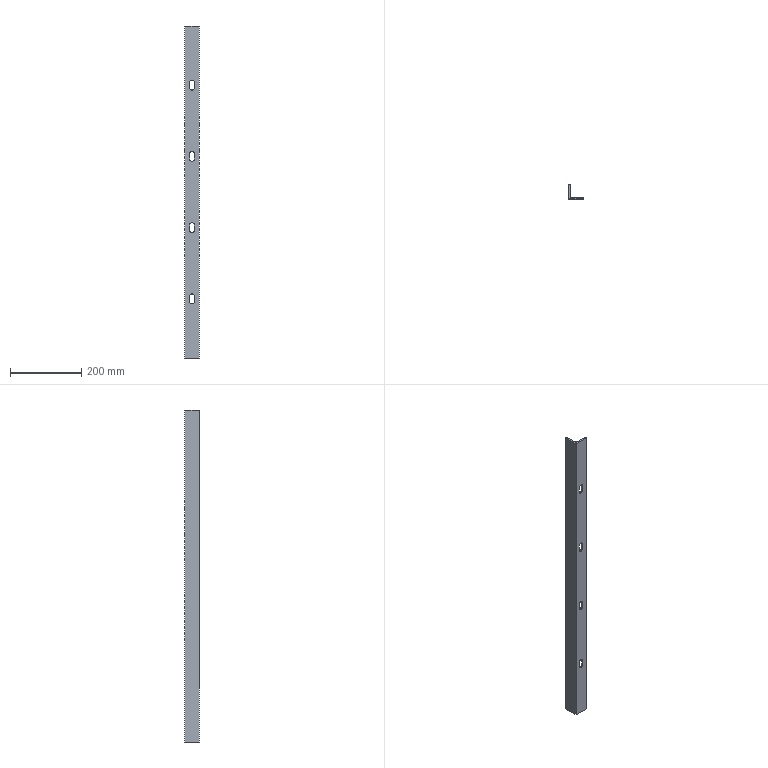Part | SolidWorks | features BaseBody 1 | 1 solid | 27 faces | box 40 x 40 x 932 mm | volume 282373 mm3 | plane 16 | cylinder 11 | commonest cylinder face diameters 13 x8 2.667 x2 10 x1
STEP:
#1=CARTESIAN_POINT('',(-11.3,51.3,0.));
#2=VERTEX_POINT('',#1);
#3=CARTESIAN_POINT('',(-11.3,11.3,0.));
#4=VERTEX_POINT('',#3);
#5=CARTESIAN_POINT('',(-11.3,11.3,0.));
#6=DIRECTION('',(0.,-1.,0.));
#7=VECTOR('',#6,1000.);
#8=LINE('',#5,#7);
#9=EDGE_CURVE('',#2,#4,#8,.T.);
#10=ORIENTED_EDGE('',*,*,#9,.T.);
#11=CARTESIAN_POINT('',(-11.3,11.3,932.));
#12=VERTEX_POINT('',#11);
#13=CARTESIAN_POINT('',(-11.3,11.3,0.));
#14=DIRECTION('',(0.,0.,1.));
#15=VECTOR('',#14,1000.);
#16=LINE('',#13,#15);
#17=EDGE_CURVE('',#4,#12,#16,.T.);
#18=ORIENTED_EDGE('',*,*,#17,.T.);
#19=CARTESIAN_POINT('',(-11.3,51.3,932.));
#20=VERTEX_POINT('',#19);
#21=CARTESIAN_POINT('',(-11.3,11.3,932.));
#22=DIRECTION('',(0.,1.,0.));
#23=VECTOR('',#22,1000.);
#24=LINE('',#21,#23);
#25=EDGE_CURVE('',#12,#20,#24,.T.);
#26=ORIENTED_EDGE('',*,*,#25,.T.);
#27=CARTESIAN_POINT('',(-11.3,51.3,0.));
#28=DIRECTION('',(0.,0.,-1.));
#29=VECTOR('',#28,1000.);
#30=LINE('',#27,#29);
#31=EDGE_CURVE('',#20,#2,#30,.T.);
#32=ORIENTED_EDGE('',*,*,#31,.T.);
#33=EDGE_LOOP('',(#10,#18,#26,#32));
#34=FACE_OUTER_BOUND('',#33,.T.);
#35=CARTESIAN_POINT('',(-11.3,11.3,0.));
#36=DIRECTION('',(-1.,0.,0.));
#37=DIRECTION('',(0.,-1.,0.));
#38=AXIS2_PLACEMENT_3D('',#35,#36,#37);
#39=PLANE('',#38);
#40=ADVANCED_FACE('',(#34),#39,.T.);
#41=CARTESIAN_POINT('',(2.2,11.3,773.5));
#42=VERTEX_POINT('',#41);
#43=CARTESIAN_POINT('',(15.2,11.3,773.5));
#44=VERTEX_POINT('',#43);
#45=CARTESIAN_POINT('',(8.7,11.3,773.5));
#46=DIRECTION('',(0.,1.,0.));
#47=DIRECTION('',(-1.,0.,0.));
#48=AXIS2_PLACEMENT_3D('',#45,#46,#47);
#49=CIRCLE('',#48,6.5);
#50=EDGE_CURVE('',#42,#44,#49,.T.);
#51=ORIENTED_EDGE('',*,*,#50,.T.);
#52=CARTESIAN_POINT('',(15.2,11.3,758.5));
#53=VERTEX_POINT('',#52);
#54=CARTESIAN_POINT('',(15.2,11.3,0.));
#55=DIRECTION('',(0.,0.,-1.));
#56=VECTOR('',#55,1000.);
#57=LINE('',#54,#56);
#58=EDGE_CURVE('',#44,#53,#57,.T.);
#59=ORIENTED_EDGE('',*,*,#58,.T.);
#60=CARTESIAN_POINT('',(2.2,11.3,758.5));
#61=VERTEX_POINT('',#60);
#62=CARTESIAN_POINT('',(8.7,11.3,758.5));
#63=DIRECTION('',(0.,1.,0.));
#64=DIRECTION('',(-1.,0.,0.));
#65=AXIS2_PLACEMENT_3D('',#62,#63,#64);
#66=CIRCLE('',#65,6.5);
#67=EDGE_CURVE('',#53,#61,#66,.T.);
#68=ORIENTED_EDGE('',*,*,#67,.T.);
#69=CARTESIAN_POINT('',(2.2,11.3,0.));
#70=DIRECTION('',(0.,0.,1.));
#71=VECTOR('',#70,1000.);
#72=LINE('',#69,#71);
#73=EDGE_CURVE('',#61,#42,#72,.T.);
#74=ORIENTED_EDGE('',*,*,#73,.T.);
#75=EDGE_LOOP('',(#51,#59,#68,#74));
#76=FACE_BOUND('',#75,.T.);
#77=CARTESIAN_POINT('',(2.2,11.3,573.5));
#78=VERTEX_POINT('',#77);
#79=CARTESIAN_POINT('',(15.2,11.3,573.5));
#80=VERTEX_POINT('',#79);
#81=CARTESIAN_POINT('',(8.7,11.3,573.5));
#82=DIRECTION('',(0.,1.,0.));
#83=DIRECTION('',(-1.,0.,0.));
#84=AXIS2_PLACEMENT_3D('',#81,#82,#83);
#85=CIRCLE('',#84,6.5);
#86=EDGE_CURVE('',#78,#80,#85,.T.);
#87=ORIENTED_EDGE('',*,*,#86,.T.);
#88=CARTESIAN_POINT('',(15.2,11.3,558.5));
#89=VERTEX_POINT('',#88);
#90=CARTESIAN_POINT('',(15.2,11.3,0.));
#91=DIRECTION('',(0.,0.,-1.));
#92=VECTOR('',#91,1000.);
#93=LINE('',#90,#92);
#94=EDGE_CURVE('',#80,#89,#93,.T.);
#95=ORIENTED_EDGE('',*,*,#94,.T.);
#96=CARTESIAN_POINT('',(2.2,11.3,558.5));
#97=VERTEX_POINT('',#96);
#98=CARTESIAN_POINT('',(8.7,11.3,558.5));
#99=DIRECTION('',(0.,1.,0.));
#100=DIRECTION('',(-1.,0.,0.));
#101=AXIS2_PLACEMENT_3D('',#98,#99,#100);
#102=CIRCLE('',#101,6.5);
#103=EDGE_CURVE('',#89,#97,#102,.T.);
#104=ORIENTED_EDGE('',*,*,#103,.T.);
#105=CARTESIAN_POINT('',(2.2,11.3,0.));
#106=DIRECTION('',(0.,0.,1.));
#107=VECTOR('',#106,1000.);
#108=LINE('',#105,#107);
#109=EDGE_CURVE('',#97,#78,#108,.T.);
#110=ORIENTED_EDGE('',*,*,#109,.T.);
#111=EDGE_LOOP('',(#87,#95,#104,#110));
#112=FACE_BOUND('',#111,.T.);
#113=CARTESIAN_POINT('',(2.2,11.3,373.5));
#114=VERTEX_POINT('',#113);
#115=CARTESIAN_POINT('',(15.2,11.3,373.5));
#116=VERTEX_POINT('',#115);
#117=CARTESIAN_POINT('',(8.7,11.3,373.5));
#118=DIRECTION('',(0.,1.,0.));
#119=DIRECTION('',(-1.,0.,0.));
#120=AXIS2_PLACEMENT_3D('',#117,#118,#119);
#121=CIRCLE('',#120,6.5);
#122=EDGE_CURVE('',#114,#116,#121,.T.);
#123=ORIENTED_EDGE('',*,*,#122,.T.);
#124=CARTESIAN_POINT('',(15.2,11.3,358.5));
#125=VERTEX_POINT('',#124);
#126=CARTESIAN_POINT('',(15.2,11.3,0.));
#127=DIRECTION('',(0.,0.,-1.));
#128=VECTOR('',#127,1000.);
#129=LINE('',#126,#128);
#130=EDGE_CURVE('',#116,#125,#129,.T.);
#131=ORIENTED_EDGE('',*,*,#130,.T.);
#132=CARTESIAN_POINT('',(2.2,11.3,358.5));
#133=VERTEX_POINT('',#132);
#134=CARTESIAN_POINT('',(8.7,11.3,358.5));
#135=DIRECTION('',(0.,1.,0.));
#136=DIRECTION('',(-1.,0.,0.));
#137=AXIS2_PLACEMENT_3D('',#134,#135,#136);
#138=CIRCLE('',#137,6.5);
#139=EDGE_CURVE('',#125,#133,#138,.T.);
#140=ORIENTED_EDGE('',*,*,#139,.T.);
#141=CARTESIAN_POINT('',(2.2,11.3,0.));
#142=DIRECTION('',(0.,0.,1.));
#143=VECTOR('',#142,1000.);
#144=LINE('',#141,#143);
#145=EDGE_CURVE('',#133,#114,#144,.T.);
#146=ORIENTED_EDGE('',*,*,#145,.T.);
#147=EDGE_LOOP('',(#123,#131,#140,#146));
#148=FACE_BOUND('',#147,.T.);
#149=CARTESIAN_POINT('',(2.2,11.3,173.5));
#150=VERTEX_POINT('',#149);
#151=CARTESIAN_POINT('',(15.2,11.3,173.5));
#152=VERTEX_POINT('',#151);
#153=CARTESIAN_POINT('',(8.7,11.3,173.5));
#154=DIRECTION('',(0.,1.,0.));
#155=DIRECTION('',(-1.,0.,0.));
#156=AXIS2_PLACEMENT_3D('',#153,#154,#155);
#157=CIRCLE('',#156,6.5);
#158=EDGE_CURVE('',#150,#152,#157,.T.);
#159=ORIENTED_EDGE('',*,*,#158,.T.);
#160=CARTESIAN_POINT('',(15.2,11.3,158.5));
#161=VERTEX_POINT('',#160);
#162=CARTESIAN_POINT('',(15.2,11.3,0.));
#163=DIRECTION('',(0.,0.,-1.));
#164=VECTOR('',#163,1000.);
#165=LINE('',#162,#164);
#166=EDGE_CURVE('',#152,#161,#165,.T.);
#167=ORIENTED_EDGE('',*,*,#166,.T.);
#168=CARTESIAN_POINT('',(2.2,11.3,158.5));
#169=VERTEX_POINT('',#168);
#170=CARTESIAN_POINT('',(8.7,11.3,158.5));
#171=DIRECTION('',(0.,1.,0.));
#172=DIRECTION('',(-1.,0.,0.));
#173=AXIS2_PLACEMENT_3D('',#170,#171,#172);
#174=CIRCLE('',#173,6.5);
#175=EDGE_CURVE('',#161,#169,#174,.T.);
#176=ORIENTED_EDGE('',*,*,#175,.T.);
#177=CARTESIAN_POINT('',(2.2,11.3,0.));
#178=DIRECTION('',(0.,0.,1.));
#179=VECTOR('',#178,1000.);
#180=LINE('',#177,#179);
#181=EDGE_CURVE('',#169,#150,#180,.T.);
#182=ORIENTED_EDGE('',*,*,#181,.T.);
#183=EDGE_LOOP('',(#159,#167,#176,#182));
#184=FACE_BOUND('',#183,.T.);
#185=CARTESIAN_POINT('',(28.7,11.3,0.));
#186=VERTEX_POINT('',#185);
#187=CARTESIAN_POINT('',(28.7,11.3,0.));
#188=DIRECTION('',(1.,0.,0.));
#189=VECTOR('',#188,1000.);
#190=LINE('',#187,#189);
#191=EDGE_CURVE('',#4,#186,#190,.T.);
#192=ORIENTED_EDGE('',*,*,#191,.T.);
#193=CARTESIAN_POINT('',(28.7,11.3,932.));
#194=VERTEX_POINT('',#193);
#195=CARTESIAN_POINT('',(28.7,11.3,0.));
#196=DIRECTION('',(0.,0.,1.));
#197=VECTOR('',#196,1000.);
#198=LINE('',#195,#197);
#199=EDGE_CURVE('',#186,#194,#198,.T.);
#200=ORIENTED_EDGE('',*,*,#199,.T.);
#201=CARTESIAN_POINT('',(28.7,11.3,932.));
#202=DIRECTION('',(-1.,0.,0.));
#203=VECTOR('',#202,1000.);
#204=LINE('',#201,#203);
#205=EDGE_CURVE('',#194,#12,#204,.T.);
#206=ORIENTED_EDGE('',*,*,#205,.T.);
#207=ORIENTED_EDGE('',*,*,#17,.F.);
#208=EDGE_LOOP('',(#192,#200,#206,#207));
#209=FACE_OUTER_BOUND('',#208,.T.);
#210=CARTESIAN_POINT('',(28.7,11.3,0.));
#211=DIRECTION('',(0.,-1.,0.));
#212=DIRECTION('',(1.,0.,0.));
#213=AXIS2_PLACEMENT_3D('',#210,#211,#212);
#214=PLANE('',#213);
#215=ADVANCED_FACE('',(#76,#112,#148,#184,#209),#214,.T.);
#216=CARTESIAN_POINT('',(-8.633,51.3,0.));
#217=VERTEX_POINT('',#216);
#218=CARTESIAN_POINT('',(8.7,51.3,0.));
#219=DIRECTION('',(-1.,0.,0.));
#220=VECTOR('',#219,1000.);
#221=LINE('',#218,#220);
#222=EDGE_CURVE('',#217,#2,#221,.T.);
#223=ORIENTED_EDGE('',*,*,#222,.F.);
#224=CARTESIAN_POINT('',(-7.3,49.967,0.));
#225=VERTEX_POINT('',#224);
#226=CARTESIAN_POINT('',(-8.633,49.967,0.));
#227=DIRECTION('',(0.,0.,1.));
#228=DIRECTION('',(1.,0.,0.));
#229=AXIS2_PLACEMENT_3D('',#226,#227,#228);
#230=CIRCLE('',#229,1.333);
#231=EDGE_CURVE('',#225,#217,#230,.T.);
#232=ORIENTED_EDGE('',*,*,#231,.F.);
#233=CARTESIAN_POINT('',(-7.3,20.3,0.));
#234=VERTEX_POINT('',#233);
#235=CARTESIAN_POINT('',(-7.3,31.3,0.));
#236=DIRECTION('',(0.,1.,0.));
#237=VECTOR('',#236,1000.);
#238=LINE('',#235,#237);
#239=EDGE_CURVE('',#234,#225,#238,.T.);
#240=ORIENTED_EDGE('',*,*,#239,.F.);
#241=CARTESIAN_POINT('',(-2.3,15.3,0.));
#242=VERTEX_POINT('',#241);
#243=CARTESIAN_POINT('',(-2.3,20.3,0.));
#244=DIRECTION('',(0.,0.,-1.));
#245=DIRECTION('',(1.,0.,0.));
#246=AXIS2_PLACEMENT_3D('',#243,#244,#245);
#247=CIRCLE('',#246,5.);
#248=EDGE_CURVE('',#242,#234,#247,.T.);
#249=ORIENTED_EDGE('',*,*,#248,.F.);
#250=CARTESIAN_POINT('',(27.367,15.3,0.));
#251=VERTEX_POINT('',#250);
#252=CARTESIAN_POINT('',(8.7,15.3,0.));
#253=DIRECTION('',(-1.,0.,0.));
#254=VECTOR('',#253,1000.);
#255=LINE('',#252,#254);
#256=EDGE_CURVE('',#251,#242,#255,.T.);
#257=ORIENTED_EDGE('',*,*,#256,.F.);
#258=CARTESIAN_POINT('',(28.7,13.967,0.));
#259=VERTEX_POINT('',#258);
#260=CARTESIAN_POINT('',(27.367,13.967,0.));
#261=DIRECTION('',(0.,0.,1.));
#262=DIRECTION('',(1.,0.,0.));
#263=AXIS2_PLACEMENT_3D('',#260,#261,#262);
#264=CIRCLE('',#263,1.333);
#265=EDGE_CURVE('',#259,#251,#264,.T.);
#266=ORIENTED_EDGE('',*,*,#265,.F.);
#267=CARTESIAN_POINT('',(28.7,31.3,0.));
#268=DIRECTION('',(0.,1.,0.));
#269=VECTOR('',#268,1000.);
#270=LINE('',#267,#269);
#271=EDGE_CURVE('',#186,#259,#270,.T.);
#272=ORIENTED_EDGE('',*,*,#271,.F.);
#273=ORIENTED_EDGE('',*,*,#191,.F.);
#274=ORIENTED_EDGE('',*,*,#9,.F.);
#275=EDGE_LOOP('',(#223,#232,#240,#249,#257,#266,#272,#273,#274));
#276=FACE_OUTER_BOUND('',#275,.T.);
#277=CARTESIAN_POINT('',(8.7,31.3,0.));
#278=DIRECTION('',(0.,0.,1.));
#279=DIRECTION('',(1.,0.,0.));
#280=AXIS2_PLACEMENT_3D('',#277,#278,#279);
#281=PLANE('',#280);
#282=ADVANCED_FACE('',(#276),#281,.F.);
#283=ORIENTED_EDGE('',*,*,#222,.T.);
#284=ORIENTED_EDGE('',*,*,#31,.F.);
#285=CARTESIAN_POINT('',(-8.633,51.3,932.));
#286=VERTEX_POINT('',#285);
#287=CARTESIAN_POINT('',(-11.3,51.3,932.));
#288=DIRECTION('',(1.,0.,0.));
#289=VECTOR('',#288,1000.);
#290=LINE('',#287,#289);
#291=EDGE_CURVE('',#20,#286,#290,.T.);
#292=ORIENTED_EDGE('',*,*,#291,.T.);
#293=CARTESIAN_POINT('',(-8.633,51.3,0.));
#294=DIRECTION('',(0.,0.,-1.));
#295=VECTOR('',#294,1000.);
#296=LINE('',#293,#295);
#297=EDGE_CURVE('',#286,#217,#296,.T.);
#298=ORIENTED_EDGE('',*,*,#297,.T.);
#299=EDGE_LOOP('',(#283,#284,#292,#298));
#300=FACE_OUTER_BOUND('',#299,.T.);
#301=CARTESIAN_POINT('',(-11.3,51.3,0.));
#302=DIRECTION('',(0.,1.,0.));
#303=DIRECTION('',(0.,0.,1.));
#304=AXIS2_PLACEMENT_3D('',#301,#302,#303);
#305=PLANE('',#304);
#306=ADVANCED_FACE('',(#300),#305,.T.);
#307=CARTESIAN_POINT('',(-7.3,49.967,932.));
#308=VERTEX_POINT('',#307);
#309=CARTESIAN_POINT('',(-8.633,49.967,932.));
#310=DIRECTION('',(0.,0.,1.));
#311=DIRECTION('',(1.,0.,0.));
#312=AXIS2_PLACEMENT_3D('',#309,#310,#311);
#313=CIRCLE('',#312,1.333);
#314=EDGE_CURVE('',#308,#286,#313,.T.);
#315=ORIENTED_EDGE('',*,*,#314,.T.);
#316=ORIENTED_EDGE('',*,*,#291,.F.);
#317=ORIENTED_EDGE('',*,*,#25,.F.);
#318=ORIENTED_EDGE('',*,*,#205,.F.);
#319=CARTESIAN_POINT('',(28.7,13.967,932.));
#320=VERTEX_POINT('',#319);
#321=CARTESIAN_POINT('',(28.7,31.3,932.));
#322=DIRECTION('',(0.,1.,0.));
#323=VECTOR('',#322,1000.);
#324=LINE('',#321,#323);
#325=EDGE_CURVE('',#194,#320,#324,.T.);
#326=ORIENTED_EDGE('',*,*,#325,.T.);
#327=CARTESIAN_POINT('',(27.367,15.3,932.));
#328=VERTEX_POINT('',#327);
#329=CARTESIAN_POINT('',(27.367,13.967,932.));
#330=DIRECTION('',(0.,0.,1.));
#331=DIRECTION('',(1.,0.,0.));
#332=AXIS2_PLACEMENT_3D('',#329,#330,#331);
#333=CIRCLE('',#332,1.333);
#334=EDGE_CURVE('',#320,#328,#333,.T.);
#335=ORIENTED_EDGE('',*,*,#334,.T.);
#336=CARTESIAN_POINT('',(-2.3,15.3,932.));
#337=VERTEX_POINT('',#336);
#338=CARTESIAN_POINT('',(8.7,15.3,932.));
#339=DIRECTION('',(-1.,0.,0.));
#340=VECTOR('',#339,1000.);
#341=LINE('',#338,#340);
#342=EDGE_CURVE('',#328,#337,#341,.T.);
#343=ORIENTED_EDGE('',*,*,#342,.T.);
#344=CARTESIAN_POINT('',(-7.3,20.3,932.));
#345=VERTEX_POINT('',#344);
#346=CARTESIAN_POINT('',(-2.3,20.3,932.));
#347=DIRECTION('',(0.,0.,-1.));
#348=DIRECTION('',(1.,0.,0.));
#349=AXIS2_PLACEMENT_3D('',#346,#347,#348);
#350=CIRCLE('',#349,5.);
#351=EDGE_CURVE('',#337,#345,#350,.T.);
#352=ORIENTED_EDGE('',*,*,#351,.T.);
#353=CARTESIAN_POINT('',(-7.3,31.3,932.));
#354=DIRECTION('',(0.,1.,0.));
#355=VECTOR('',#354,1000.);
#356=LINE('',#353,#355);
#357=EDGE_CURVE('',#345,#308,#356,.T.);
#358=ORIENTED_EDGE('',*,*,#357,.T.);
#359=EDGE_LOOP('',(#315,#316,#317,#318,#326,#335,#343,#352,#358));
#360=FACE_OUTER_BOUND('',#359,.T.);
#361=CARTESIAN_POINT('',(8.7,31.3,932.));
#362=DIRECTION('',(0.,0.,1.));
#363=DIRECTION('',(1.,0.,0.));
#364=AXIS2_PLACEMENT_3D('',#361,#362,#363);
#365=PLANE('',#364);
#366=ADVANCED_FACE('',(#360),#365,.T.);
#367=CARTESIAN_POINT('',(15.2,15.3,758.5));
#368=VERTEX_POINT('',#367);
#369=CARTESIAN_POINT('',(15.2,11.3,758.5));
#370=DIRECTION('',(0.,1.,0.));
#371=VECTOR('',#370,1000.);
#372=LINE('',#369,#371);
#373=EDGE_CURVE('',#53,#368,#372,.T.);
#374=ORIENTED_EDGE('',*,*,#373,.F.);
#375=ORIENTED_EDGE('',*,*,#58,.F.);
#376=CARTESIAN_POINT('',(15.2,15.3,773.5));
#377=VERTEX_POINT('',#376);
#378=CARTESIAN_POINT('',(15.2,11.3,773.5));
#379=DIRECTION('',(0.,-1.,0.));
#380=VECTOR('',#379,1000.);
#381=LINE('',#378,#380);
#382=EDGE_CURVE('',#377,#44,#381,.T.);
#383=ORIENTED_EDGE('',*,*,#382,.F.);
#384=CARTESIAN_POINT('',(15.2,15.3,773.5));
#385=DIRECTION('',(0.,0.,1.));
#386=VECTOR('',#385,1000.);
#387=LINE('',#384,#386);
#388=EDGE_CURVE('',#368,#377,#387,.T.);
#389=ORIENTED_EDGE('',*,*,#388,.F.);
#390=EDGE_LOOP('',(#374,#375,#383,#389));
#391=FACE_OUTER_BOUND('',#390,.T.);
#392=CARTESIAN_POINT('',(15.2,11.3,773.5));
#393=DIRECTION('',(1.,0.,0.));
#394=DIRECTION('',(0.,1.,0.));
#395=AXIS2_PLACEMENT_3D('',#392,#393,#394);
#396=PLANE('',#395);
#397=ADVANCED_FACE('',(#391),#396,.F.);
#398=ORIENTED_EDGE('',*,*,#382,.T.);
#399=ORIENTED_EDGE('',*,*,#50,.F.);
#400=CARTESIAN_POINT('',(2.2,15.3,773.5));
#401=VERTEX_POINT('',#400);
#402=CARTESIAN_POINT('',(2.2,11.3,773.5));
#403=DIRECTION('',(0.,-1.,0.));
#404=VECTOR('',#403,1000.);
#405=LINE('',#402,#404);
#406=EDGE_CURVE('',#401,#42,#405,.T.);
#407=ORIENTED_EDGE('',*,*,#406,.F.);
#408=CARTESIAN_POINT('',(8.7,15.3,773.5));
#409=DIRECTION('',(0.,-1.,0.));
#410=DIRECTION('',(-1.,0.,0.));
#411=AXIS2_PLACEMENT_3D('',#408,#409,#410);
#412=CIRCLE('',#411,6.5);
#413=EDGE_CURVE('',#377,#401,#412,.T.);
#414=ORIENTED_EDGE('',*,*,#413,.F.);
#415=EDGE_LOOP('',(#398,#399,#407,#414));
#416=FACE_OUTER_BOUND('',#415,.T.);
#417=CARTESIAN_POINT('',(8.7,11.3,773.5));
#418=DIRECTION('',(0.,1.,0.));
#419=DIRECTION('',(-1.,0.,0.));
#420=AXIS2_PLACEMENT_3D('',#417,#418,#419);
#421=CYLINDRICAL_SURFACE('',#420,6.5);
#422=ADVANCED_FACE('',(#416),#421,.F.);
#423=ORIENTED_EDGE('',*,*,#406,.T.);
#424=ORIENTED_EDGE('',*,*,#73,.F.);
#425=CARTESIAN_POINT('',(2.2,15.3,758.5));
#426=VERTEX_POINT('',#425);
#427=CARTESIAN_POINT('',(2.2,11.3,758.5));
#428=DIRECTION('',(0.,-1.,0.));
#429=VECTOR('',#428,1000.);
#430=LINE('',#427,#429);
#431=EDGE_CURVE('',#426,#61,#430,.T.);
#432=ORIENTED_EDGE('',*,*,#431,.F.);
#433=CARTESIAN_POINT('',(2.2,15.3,758.5));
#434=DIRECTION('',(0.,0.,-1.));
#435=VECTOR('',#434,1000.);
#436=LINE('',#433,#435);
#437=EDGE_CURVE('',#401,#426,#436,.T.);
#438=ORIENTED_EDGE('',*,*,#437,.F.);
#439=EDGE_LOOP('',(#423,#424,#432,#438));
#440=FACE_OUTER_BOUND('',#439,.T.);
#441=CARTESIAN_POINT('',(2.2,11.3,758.5));
#442=DIRECTION('',(-1.,0.,0.));
#443=DIRECTION('',(0.,0.,1.));
#444=AXIS2_PLACEMENT_3D('',#441,#442,#443);
#445=PLANE('',#444);
#446=ADVANCED_FACE('',(#440),#445,.F.);
#447=ORIENTED_EDGE('',*,*,#431,.T.);
#448=ORIENTED_EDGE('',*,*,#67,.F.);
#449=ORIENTED_EDGE('',*,*,#373,.T.);
#450=CARTESIAN_POINT('',(8.7,15.3,758.5));
#451=DIRECTION('',(0.,-1.,0.));
#452=DIRECTION('',(-1.,0.,0.));
#453=AXIS2_PLACEMENT_3D('',#450,#451,#452);
#454=CIRCLE('',#453,6.5);
#455=EDGE_CURVE('',#426,#368,#454,.T.);
#456=ORIENTED_EDGE('',*,*,#455,.F.);
#457=EDGE_LOOP('',(#447,#448,#449,#456));
#458=FACE_OUTER_BOUND('',#457,.T.);
#459=CARTESIAN_POINT('',(8.7,11.3,758.5));
#460=DIRECTION('',(0.,1.,0.));
#461=DIRECTION('',(-1.,0.,0.));
#462=AXIS2_PLACEMENT_3D('',#459,#460,#461);
#463=CYLINDRICAL_SURFACE('',#462,6.5);
#464=ADVANCED_FACE('',(#458),#463,.F.);
#465=CARTESIAN_POINT('',(15.2,15.3,558.5));
#466=VERTEX_POINT('',#465);
#467=CARTESIAN_POINT('',(15.2,11.3,558.5));
#468=DIRECTION('',(0.,1.,0.));
#469=VECTOR('',#468,1000.);
#470=LINE('',#467,#469);
#471=EDGE_CURVE('',#89,#466,#470,.T.);
#472=ORIENTED_EDGE('',*,*,#471,.F.);
#473=ORIENTED_EDGE('',*,*,#94,.F.);
#474=CARTESIAN_POINT('',(15.2,15.3,573.5));
#475=VERTEX_POINT('',#474);
#476=CARTESIAN_POINT('',(15.2,11.3,573.5));
#477=DIRECTION('',(0.,-1.,0.));
#478=VECTOR('',#477,1000.);
#479=LINE('',#476,#478);
#480=EDGE_CURVE('',#475,#80,#479,.T.);
#481=ORIENTED_EDGE('',*,*,#480,.F.);
#482=CARTESIAN_POINT('',(15.2,15.3,573.5));
#483=DIRECTION('',(0.,0.,1.));
#484=VECTOR('',#483,1000.);
#485=LINE('',#482,#484);
#486=EDGE_CURVE('',#466,#475,#485,.T.);
#487=ORIENTED_EDGE('',*,*,#486,.F.);
#488=EDGE_LOOP('',(#472,#473,#481,#487));
#489=FACE_OUTER_BOUND('',#488,.T.);
#490=CARTESIAN_POINT('',(15.2,11.3,573.5));
#491=DIRECTION('',(1.,0.,0.));
#492=DIRECTION('',(0.,1.,0.));
#493=AXIS2_PLACEMENT_3D('',#490,#491,#492);
#494=PLANE('',#493);
#495=ADVANCED_FACE('',(#489),#494,.F.);
#496=ORIENTED_EDGE('',*,*,#480,.T.);
#497=ORIENTED_EDGE('',*,*,#86,.F.);
#498=CARTESIAN_POINT('',(2.2,15.3,573.5));
#499=VERTEX_POINT('',#498);
#500=CARTESIAN_POINT('',(2.2,11.3,573.5));
#501=DIRECTION('',(0.,-1.,0.));
#502=VECTOR('',#501,1000.);
#503=LINE('',#500,#502);
#504=EDGE_CURVE('',#499,#78,#503,.T.);
#505=ORIENTED_EDGE('',*,*,#504,.F.);
#506=CARTESIAN_POINT('',(8.7,15.3,573.5));
#507=DIRECTION('',(0.,-1.,0.));
#508=DIRECTION('',(-1.,0.,0.));
#509=AXIS2_PLACEMENT_3D('',#506,#507,#508);
#510=CIRCLE('',#509,6.5);
#511=EDGE_CURVE('',#475,#499,#510,.T.);
#512=ORIENTED_EDGE('',*,*,#511,.F.);
#513=EDGE_LOOP('',(#496,#497,#505,#512));
#514=FACE_OUTER_BOUND('',#513,.T.);
#515=CARTESIAN_POINT('',(8.7,11.3,573.5));
#516=DIRECTION('',(0.,1.,0.));
#517=DIRECTION('',(-1.,0.,0.));
#518=AXIS2_PLACEMENT_3D('',#515,#516,#517);
#519=CYLINDRICAL_SURFACE('',#518,6.5);
#520=ADVANCED_FACE('',(#514),#519,.F.);
#521=ORIENTED_EDGE('',*,*,#504,.T.);
#522=ORIENTED_EDGE('',*,*,#109,.F.);
#523=CARTESIAN_POINT('',(2.2,15.3,558.5));
#524=VERTEX_POINT('',#523);
#525=CARTESIAN_POINT('',(2.2,11.3,558.5));
#526=DIRECTION('',(0.,-1.,0.));
#527=VECTOR('',#526,1000.);
#528=LINE('',#525,#527);
#529=EDGE_CURVE('',#524,#97,#528,.T.);
#530=ORIENTED_EDGE('',*,*,#529,.F.);
#531=CARTESIAN_POINT('',(2.2,15.3,558.5));
#532=DIRECTION('',(0.,0.,-1.));
#533=VECTOR('',#532,1000.);
#534=LINE('',#531,#533);
#535=EDGE_CURVE('',#499,#524,#534,.T.);
#536=ORIENTED_EDGE('',*,*,#535,.F.);
#537=EDGE_LOOP('',(#521,#522,#530,#536));
#538=FACE_OUTER_BOUND('',#537,.T.);
#539=CARTESIAN_POINT('',(2.2,11.3,558.5));
#540=DIRECTION('',(-1.,0.,0.));
#541=DIRECTION('',(0.,0.,1.));
#542=AXIS2_PLACEMENT_3D('',#539,#540,#541);
#543=PLANE('',#542);
#544=ADVANCED_FACE('',(#538),#543,.F.);
#545=ORIENTED_EDGE('',*,*,#529,.T.);
#546=ORIENTED_EDGE('',*,*,#103,.F.);
#547=ORIENTED_EDGE('',*,*,#471,.T.);
#548=CARTESIAN_POINT('',(8.7,15.3,558.5));
#549=DIRECTION('',(0.,-1.,0.));
#550=DIRECTION('',(-1.,0.,0.));
#551=AXIS2_PLACEMENT_3D('',#548,#549,#550);
#552=CIRCLE('',#551,6.5);
#553=EDGE_CURVE('',#524,#466,#552,.T.);
#554=ORIENTED_EDGE('',*,*,#553,.F.);
#555=EDGE_LOOP('',(#545,#546,#547,#554));
#556=FACE_OUTER_BOUND('',#555,.T.);
#557=CARTESIAN_POINT('',(8.7,11.3,558.5));
#558=DIRECTION('',(0.,1.,0.));
#559=DIRECTION('',(-1.,0.,0.));
#560=AXIS2_PLACEMENT_3D('',#557,#558,#559);
#561=CYLINDRICAL_SURFACE('',#560,6.5);
#562=ADVANCED_FACE('',(#556),#561,.F.);
#563=CARTESIAN_POINT('',(15.2,15.3,358.5));
#564=VERTEX_POINT('',#563);
#565=CARTESIAN_POINT('',(15.2,11.3,358.5));
#566=DIRECTION('',(0.,1.,0.));
#567=VECTOR('',#566,1000.);
#568=LINE('',#565,#567);
#569=EDGE_CURVE('',#125,#564,#568,.T.);
#570=ORIENTED_EDGE('',*,*,#569,.F.);
#571=ORIENTED_EDGE('',*,*,#130,.F.);
#572=CARTESIAN_POINT('',(15.2,15.3,373.5));
#573=VERTEX_POINT('',#572);
#574=CARTESIAN_POINT('',(15.2,11.3,373.5));
#575=DIRECTION('',(0.,-1.,0.));
#576=VECTOR('',#575,1000.);
#577=LINE('',#574,#576);
#578=EDGE_CURVE('',#573,#116,#577,.T.);
#579=ORIENTED_EDGE('',*,*,#578,.F.);
#580=CARTESIAN_POINT('',(15.2,15.3,373.5));
#581=DIRECTION('',(0.,0.,1.));
#582=VECTOR('',#581,1000.);
#583=LINE('',#580,#582);
#584=EDGE_CURVE('',#564,#573,#583,.T.);
#585=ORIENTED_EDGE('',*,*,#584,.F.);
#586=EDGE_LOOP('',(#570,#571,#579,#585));
#587=FACE_OUTER_BOUND('',#586,.T.);
#588=CARTESIAN_POINT('',(15.2,11.3,373.5));
#589=DIRECTION('',(1.,0.,0.));
#590=DIRECTION('',(0.,1.,0.));
#591=AXIS2_PLACEMENT_3D('',#588,#589,#590);
#592=PLANE('',#591);
#593=ADVANCED_FACE('',(#587),#592,.F.);
#594=ORIENTED_EDGE('',*,*,#578,.T.);
#595=ORIENTED_EDGE('',*,*,#122,.F.);
#596=CARTESIAN_POINT('',(2.2,15.3,373.5));
#597=VERTEX_POINT('',#596);
#598=CARTESIAN_POINT('',(2.2,11.3,373.5));
#599=DIRECTION('',(0.,-1.,0.));
#600=VECTOR('',#599,1000.);
#601=LINE('',#598,#600);
#602=EDGE_CURVE('',#597,#114,#601,.T.);
#603=ORIENTED_EDGE('',*,*,#602,.F.);
#604=CARTESIAN_POINT('',(8.7,15.3,373.5));
#605=DIRECTION('',(0.,-1.,0.));
#606=DIRECTION('',(-1.,0.,0.));
#607=AXIS2_PLACEMENT_3D('',#604,#605,#606);
#608=CIRCLE('',#607,6.5);
#609=EDGE_CURVE('',#573,#597,#608,.T.);
#610=ORIENTED_EDGE('',*,*,#609,.F.);
#611=EDGE_LOOP('',(#594,#595,#603,#610));
#612=FACE_OUTER_BOUND('',#611,.T.);
#613=CARTESIAN_POINT('',(8.7,11.3,373.5));
#614=DIRECTION('',(0.,1.,0.));
#615=DIRECTION('',(-1.,0.,0.));
#616=AXIS2_PLACEMENT_3D('',#613,#614,#615);
#617=CYLINDRICAL_SURFACE('',#616,6.5);
#618=ADVANCED_FACE('',(#612),#617,.F.);
#619=ORIENTED_EDGE('',*,*,#602,.T.);
#620=ORIENTED_EDGE('',*,*,#145,.F.);
#621=CARTESIAN_POINT('',(2.2,15.3,358.5));
#622=VERTEX_POINT('',#621);
#623=CARTESIAN_POINT('',(2.2,11.3,358.5));
#624=DIRECTION('',(0.,-1.,0.));
#625=VECTOR('',#624,1000.);
#626=LINE('',#623,#625);
#627=EDGE_CURVE('',#622,#133,#626,.T.);
#628=ORIENTED_EDGE('',*,*,#627,.F.);
#629=CARTESIAN_POINT('',(2.2,15.3,358.5));
#630=DIRECTION('',(0.,0.,-1.));
#631=VECTOR('',#630,1000.);
#632=LINE('',#629,#631);
#633=EDGE_CURVE('',#597,#622,#632,.T.);
#634=ORIENTED_EDGE('',*,*,#633,.F.);
#635=EDGE_LOOP('',(#619,#620,#628,#634));
#636=FACE_OUTER_BOUND('',#635,.T.);
#637=CARTESIAN_POINT('',(2.2,11.3,358.5));
#638=DIRECTION('',(-1.,0.,0.));
#639=DIRECTION('',(0.,0.,1.));
#640=AXIS2_PLACEMENT_3D('',#637,#638,#639);
#641=PLANE('',#640);
#642=ADVANCED_FACE('',(#636),#641,.F.);
#643=ORIENTED_EDGE('',*,*,#627,.T.);
#644=ORIENTED_EDGE('',*,*,#139,.F.);
#645=ORIENTED_EDGE('',*,*,#569,.T.);
#646=CARTESIAN_POINT('',(8.7,15.3,358.5));
#647=DIRECTION('',(0.,-1.,0.));
#648=DIRECTION('',(-1.,0.,0.));
#649=AXIS2_PLACEMENT_3D('',#646,#647,#648);
#650=CIRCLE('',#649,6.5);
#651=EDGE_CURVE('',#622,#564,#650,.T.);
#652=ORIENTED_EDGE('',*,*,#651,.F.);
#653=EDGE_LOOP('',(#643,#644,#645,#652));
#654=FACE_OUTER_BOUND('',#653,.T.);
#655=CARTESIAN_POINT('',(8.7,11.3,358.5));
#656=DIRECTION('',(0.,1.,0.));
#657=DIRECTION('',(-1.,0.,0.));
#658=AXIS2_PLACEMENT_3D('',#655,#656,#657);
#659=CYLINDRICAL_SURFACE('',#658,6.5);
#660=ADVANCED_FACE('',(#654),#659,.F.);
#661=CARTESIAN_POINT('',(15.2,15.3,158.5));
#662=VERTEX_POINT('',#661);
#663=CARTESIAN_POINT('',(15.2,11.3,158.5));
#664=DIRECTION('',(0.,1.,0.));
#665=VECTOR('',#664,1000.);
#666=LINE('',#663,#665);
#667=EDGE_CURVE('',#161,#662,#666,.T.);
#668=ORIENTED_EDGE('',*,*,#667,.F.);
#669=ORIENTED_EDGE('',*,*,#166,.F.);
#670=CARTESIAN_POINT('',(15.2,15.3,173.5));
#671=VERTEX_POINT('',#670);
#672=CARTESIAN_POINT('',(15.2,11.3,173.5));
#673=DIRECTION('',(0.,-1.,0.));
#674=VECTOR('',#673,1000.);
#675=LINE('',#672,#674);
#676=EDGE_CURVE('',#671,#152,#675,.T.);
#677=ORIENTED_EDGE('',*,*,#676,.F.);
#678=CARTESIAN_POINT('',(15.2,15.3,173.5));
#679=DIRECTION('',(0.,0.,1.));
#680=VECTOR('',#679,1000.);
#681=LINE('',#678,#680);
#682=EDGE_CURVE('',#662,#671,#681,.T.);
#683=ORIENTED_EDGE('',*,*,#682,.F.);
#684=EDGE_LOOP('',(#668,#669,#677,#683));
#685=FACE_OUTER_BOUND('',#684,.T.);
#686=CARTESIAN_POINT('',(15.2,11.3,173.5));
#687=DIRECTION('',(1.,0.,0.));
#688=DIRECTION('',(0.,1.,0.));
#689=AXIS2_PLACEMENT_3D('',#686,#687,#688);
#690=PLANE('',#689);
#691=ADVANCED_FACE('',(#685),#690,.F.);
#692=ORIENTED_EDGE('',*,*,#676,.T.);
#693=ORIENTED_EDGE('',*,*,#158,.F.);
#694=CARTESIAN_POINT('',(2.2,15.3,173.5));
#695=VERTEX_POINT('',#694);
#696=CARTESIAN_POINT('',(2.2,11.3,173.5));
#697=DIRECTION('',(0.,-1.,0.));
#698=VECTOR('',#697,1000.);
#699=LINE('',#696,#698);
#700=EDGE_CURVE('',#695,#150,#699,.T.);
#701=ORIENTED_EDGE('',*,*,#700,.F.);
#702=CARTESIAN_POINT('',(8.7,15.3,173.5));
#703=DIRECTION('',(0.,-1.,0.));
#704=DIRECTION('',(-1.,0.,0.));
#705=AXIS2_PLACEMENT_3D('',#702,#703,#704);
#706=CIRCLE('',#705,6.5);
#707=EDGE_CURVE('',#671,#695,#706,.T.);
#708=ORIENTED_EDGE('',*,*,#707,.F.);
#709=EDGE_LOOP('',(#692,#693,#701,#708));
#710=FACE_OUTER_BOUND('',#709,.T.);
#711=CARTESIAN_POINT('',(8.7,11.3,173.5));
#712=DIRECTION('',(0.,1.,0.));
#713=DIRECTION('',(-1.,0.,0.));
#714=AXIS2_PLACEMENT_3D('',#711,#712,#713);
#715=CYLINDRICAL_SURFACE('',#714,6.5);
#716=ADVANCED_FACE('',(#710),#715,.F.);
#717=ORIENTED_EDGE('',*,*,#700,.T.);
#718=ORIENTED_EDGE('',*,*,#181,.F.);
#719=CARTESIAN_POINT('',(2.2,15.3,158.5));
#720=VERTEX_POINT('',#719);
#721=CARTESIAN_POINT('',(2.2,11.3,158.5));
#722=DIRECTION('',(0.,-1.,0.));
#723=VECTOR('',#722,1000.);
#724=LINE('',#721,#723);
#725=EDGE_CURVE('',#720,#169,#724,.T.);
#726=ORIENTED_EDGE('',*,*,#725,.F.);
#727=CARTESIAN_POINT('',(2.2,15.3,158.5));
#728=DIRECTION('',(0.,0.,-1.));
#729=VECTOR('',#728,1000.);
#730=LINE('',#727,#729);
#731=EDGE_CURVE('',#695,#720,#730,.T.);
#732=ORIENTED_EDGE('',*,*,#731,.F.);
#733=EDGE_LOOP('',(#717,#718,#726,#732));
#734=FACE_OUTER_BOUND('',#733,.T.);
#735=CARTESIAN_POINT('',(2.2,11.3,158.5));
#736=DIRECTION('',(-1.,0.,0.));
#737=DIRECTION('',(0.,0.,1.));
#738=AXIS2_PLACEMENT_3D('',#735,#736,#737);
#739=PLANE('',#738);
#740=ADVANCED_FACE('',(#734),#739,.F.);
#741=ORIENTED_EDGE('',*,*,#725,.T.);
#742=ORIENTED_EDGE('',*,*,#175,.F.);
#743=ORIENTED_EDGE('',*,*,#667,.T.);
#744=CARTESIAN_POINT('',(8.7,15.3,158.5));
#745=DIRECTION('',(0.,-1.,0.));
#746=DIRECTION('',(-1.,0.,0.));
#747=AXIS2_PLACEMENT_3D('',#744,#745,#746);
#748=CIRCLE('',#747,6.5);
#749=EDGE_CURVE('',#720,#662,#748,.T.);
#750=ORIENTED_EDGE('',*,*,#749,.F.);
#751=EDGE_LOOP('',(#741,#742,#743,#750));
#752=FACE_OUTER_BOUND('',#751,.T.);
#753=CARTESIAN_POINT('',(8.7,11.3,158.5));
#754=DIRECTION('',(0.,1.,0.));
#755=DIRECTION('',(-1.,0.,0.));
#756=AXIS2_PLACEMENT_3D('',#753,#754,#755);
#757=CYLINDRICAL_SURFACE('',#756,6.5);
#758=ADVANCED_FACE('',(#752),#757,.F.);
#759=ORIENTED_EDGE('',*,*,#271,.T.);
#760=CARTESIAN_POINT('',(28.7,13.967,0.));
#761=DIRECTION('',(0.,0.,1.));
#762=VECTOR('',#761,1000.);
#763=LINE('',#760,#762);
#764=EDGE_CURVE('',#259,#320,#763,.T.);
#765=ORIENTED_EDGE('',*,*,#764,.T.);
#766=ORIENTED_EDGE('',*,*,#325,.F.);
#767=ORIENTED_EDGE('',*,*,#199,.F.);
#768=EDGE_LOOP('',(#759,#765,#766,#767));
#769=FACE_OUTER_BOUND('',#768,.T.);
#770=CARTESIAN_POINT('',(28.7,13.967,0.));
#771=DIRECTION('',(1.,0.,0.));
#772=DIRECTION('',(0.,1.,0.));
#773=AXIS2_PLACEMENT_3D('',#770,#771,#772);
#774=PLANE('',#773);
#775=ADVANCED_FACE('',(#769),#774,.T.);
#776=ORIENTED_EDGE('',*,*,#231,.T.);
#777=ORIENTED_EDGE('',*,*,#297,.F.);
#778=ORIENTED_EDGE('',*,*,#314,.F.);
#779=CARTESIAN_POINT('',(-7.3,49.967,0.));
#780=DIRECTION('',(0.,0.,-1.));
#781=VECTOR('',#780,1000.);
#782=LINE('',#779,#781);
#783=EDGE_CURVE('',#308,#225,#782,.T.);
#784=ORIENTED_EDGE('',*,*,#783,.T.);
#785=EDGE_LOOP('',(#776,#777,#778,#784));
#786=FACE_OUTER_BOUND('',#785,.T.);
#787=CARTESIAN_POINT('',(-8.633,49.967,0.));
#788=DIRECTION('',(0.,0.,1.));
#789=DIRECTION('',(1.,0.,0.));
#790=AXIS2_PLACEMENT_3D('',#787,#788,#789);
#791=CYLINDRICAL_SURFACE('',#790,1.333);
#792=ADVANCED_FACE('',(#786),#791,.T.);
#793=ORIENTED_EDGE('',*,*,#239,.T.);
#794=ORIENTED_EDGE('',*,*,#783,.F.);
#795=ORIENTED_EDGE('',*,*,#357,.F.);
#796=CARTESIAN_POINT('',(-7.3,20.3,0.));
#797=DIRECTION('',(0.,0.,-1.));
#798=VECTOR('',#797,1000.);
#799=LINE('',#796,#798);
#800=EDGE_CURVE('',#345,#234,#799,.T.);
#801=ORIENTED_EDGE('',*,*,#800,.T.);
#802=EDGE_LOOP('',(#793,#794,#795,#801));
#803=FACE_OUTER_BOUND('',#802,.T.);
#804=CARTESIAN_POINT('',(-7.3,49.967,0.));
#805=DIRECTION('',(1.,0.,0.));
#806=DIRECTION('',(0.,1.,0.));
#807=AXIS2_PLACEMENT_3D('',#804,#805,#806);
#808=PLANE('',#807);
#809=ADVANCED_FACE('',(#803),#808,.T.);
#810=CARTESIAN_POINT('',(-2.3,15.3,0.));
#811=DIRECTION('',(0.,0.,1.));
#812=VECTOR('',#811,1000.);
#813=LINE('',#810,#812);
#814=EDGE_CURVE('',#242,#337,#813,.T.);
#815=ORIENTED_EDGE('',*,*,#814,.F.);
#816=ORIENTED_EDGE('',*,*,#248,.T.);
#817=ORIENTED_EDGE('',*,*,#800,.F.);
#818=ORIENTED_EDGE('',*,*,#351,.F.);
#819=EDGE_LOOP('',(#815,#816,#817,#818));
#820=FACE_OUTER_BOUND('',#819,.T.);
#821=CARTESIAN_POINT('',(-2.3,20.3,0.));
#822=DIRECTION('',(0.,0.,1.));
#823=DIRECTION('',(1.,0.,0.));
#824=AXIS2_PLACEMENT_3D('',#821,#822,#823);
#825=CYLINDRICAL_SURFACE('',#824,5.);
#826=ADVANCED_FACE('',(#820),#825,.F.);
#827=ORIENTED_EDGE('',*,*,#413,.T.);
#828=ORIENTED_EDGE('',*,*,#437,.T.);
#829=ORIENTED_EDGE('',*,*,#455,.T.);
#830=ORIENTED_EDGE('',*,*,#388,.T.);
#831=EDGE_LOOP('',(#827,#828,#829,#830));
#832=FACE_BOUND('',#831,.T.);
#833=ORIENTED_EDGE('',*,*,#511,.T.);
#834=ORIENTED_EDGE('',*,*,#535,.T.);
#835=ORIENTED_EDGE('',*,*,#553,.T.);
#836=ORIENTED_EDGE('',*,*,#486,.T.);
#837=EDGE_LOOP('',(#833,#834,#835,#836));
#838=FACE_BOUND('',#837,.T.);
#839=ORIENTED_EDGE('',*,*,#609,.T.);
#840=ORIENTED_EDGE('',*,*,#633,.T.);
#841=ORIENTED_EDGE('',*,*,#651,.T.);
#842=ORIENTED_EDGE('',*,*,#584,.T.);
#843=EDGE_LOOP('',(#839,#840,#841,#842));
#844=FACE_BOUND('',#843,.T.);
#845=ORIENTED_EDGE('',*,*,#707,.T.);
#846=ORIENTED_EDGE('',*,*,#731,.T.);
#847=ORIENTED_EDGE('',*,*,#749,.T.);
#848=ORIENTED_EDGE('',*,*,#682,.T.);
#849=EDGE_LOOP('',(#845,#846,#847,#848));
#850=FACE_BOUND('',#849,.T.);
#851=ORIENTED_EDGE('',*,*,#256,.T.);
#852=ORIENTED_EDGE('',*,*,#814,.T.);
#853=ORIENTED_EDGE('',*,*,#342,.F.);
#854=CARTESIAN_POINT('',(27.367,15.3,0.));
#855=DIRECTION('',(0.,0.,-1.));
#856=VECTOR('',#855,1000.);
#857=LINE('',#854,#856);
#858=EDGE_CURVE('',#328,#251,#857,.T.);
#859=ORIENTED_EDGE('',*,*,#858,.T.);
#860=EDGE_LOOP('',(#851,#852,#853,#859));
#861=FACE_OUTER_BOUND('',#860,.T.);
#862=CARTESIAN_POINT('',(-2.3,15.3,0.));
#863=DIRECTION('',(0.,1.,0.));
#864=DIRECTION('',(-1.,0.,0.));
#865=AXIS2_PLACEMENT_3D('',#862,#863,#864);
#866=PLANE('',#865);
#867=ADVANCED_FACE('',(#832,#838,#844,#850,#861),#866,.T.);
#868=ORIENTED_EDGE('',*,*,#265,.T.);
#869=ORIENTED_EDGE('',*,*,#858,.F.);
#870=ORIENTED_EDGE('',*,*,#334,.F.);
#871=ORIENTED_EDGE('',*,*,#764,.F.);
#872=EDGE_LOOP('',(#868,#869,#870,#871));
#873=FACE_OUTER_BOUND('',#872,.T.);
#874=CARTESIAN_POINT('',(27.367,13.967,0.));
#875=DIRECTION('',(0.,0.,1.));
#876=DIRECTION('',(1.,0.,0.));
#877=AXIS2_PLACEMENT_3D('',#874,#875,#876);
#878=CYLINDRICAL_SURFACE('',#877,1.333);
#879=ADVANCED_FACE('',(#873),#878,.T.);
#880=CLOSED_SHELL('',(#40,#215,#282,#306,#366,#397,#422,#446,#464,#495,#520,#544,#562,#593,#618,#642,#660,#691,#716,#740,#758,#775,#792,#809,#826,#867,#879));
#881=MANIFOLD_SOLID_BREP('',#880);
#882=CARTESIAN_POINT('',(0.,0.,0.));
#883=DIRECTION('',(0.,0.,1.));
#884=DIRECTION('',(1.,0.,0.));
#885=AXIS2_PLACEMENT_3D('',#882,#883,#884);
#886=(LENGTH_UNIT()NAMED_UNIT(*)SI_UNIT(.MILLI.,.METRE.));
#887=UNCERTAINTY_MEASURE_WITH_UNIT(LENGTH_MEASURE(0.00001),#886,'','');
#888=(NAMED_UNIT(*)PLANE_ANGLE_UNIT()SI_UNIT($,.RADIAN.));
#889=(NAMED_UNIT(*)SI_UNIT($,.STERADIAN.)SOLID_ANGLE_UNIT());
#890=(GEOMETRIC_REPRESENTATION_CONTEXT(3)GLOBAL_UNCERTAINTY_ASSIGNED_CONTEXT((#887))GLOBAL_UNIT_ASSIGNED_CONTEXT((#886,#888,#889))REPRESENTATION_CONTEXT('',''));
#891=ADVANCED_BREP_SHAPE_REPRESENTATION('',(#881,#885),#890);